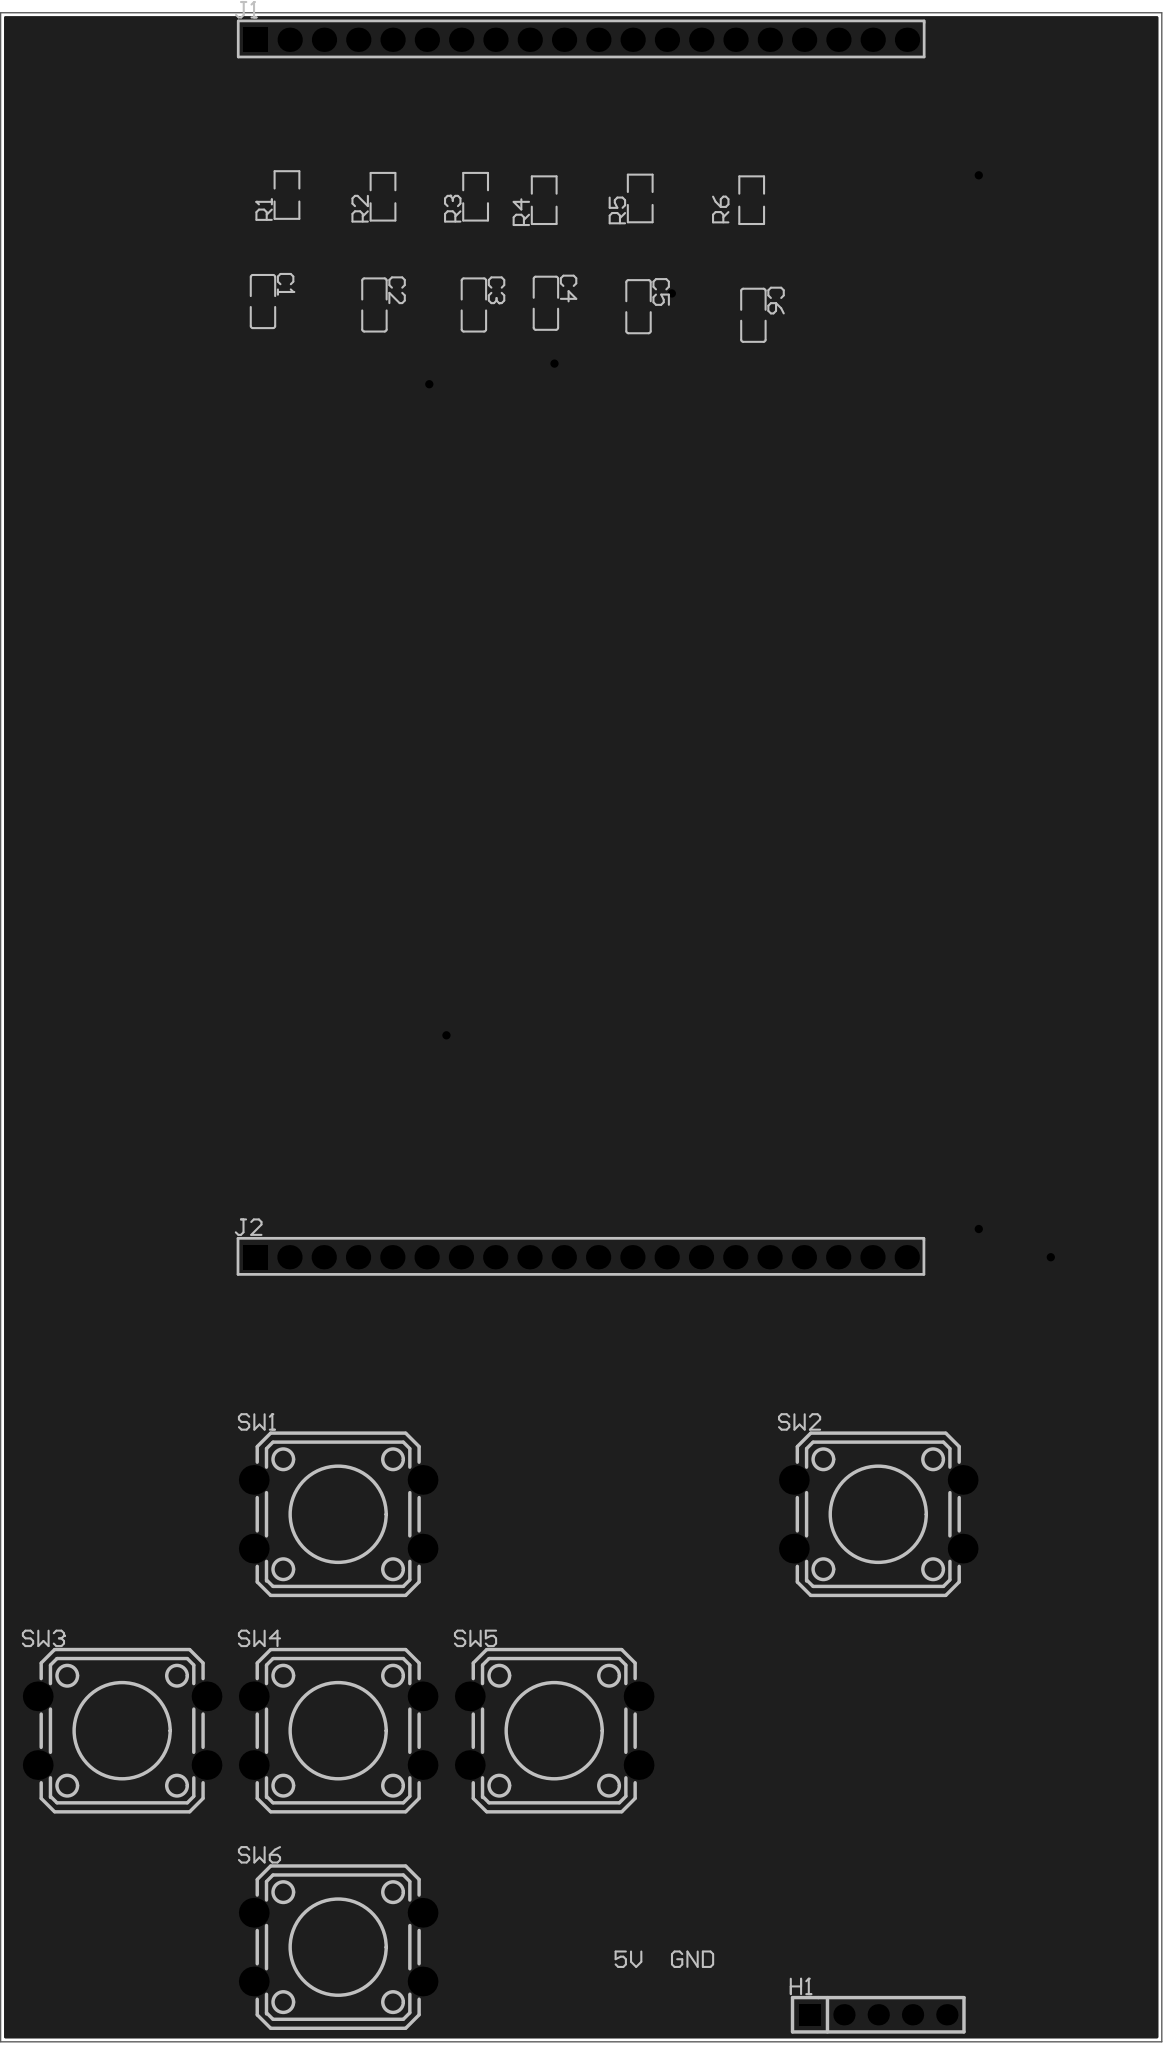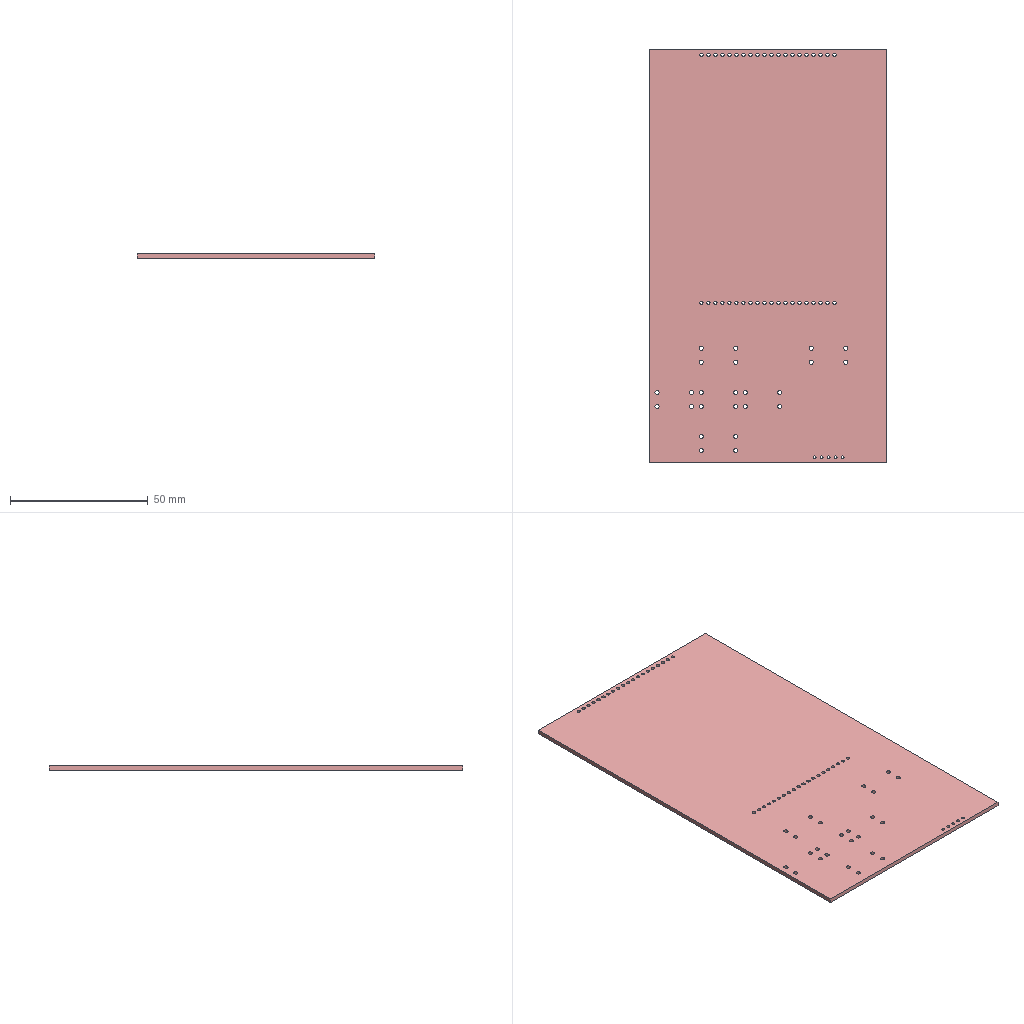Circuit board layout | Altium Designer | box 86 x 150 x 1.6 mm
Layer stack:
# Altium Designer layer stack of  (unit mm; dielectric type: 0 none, 1 core, 2 prepreg, 3 surface material)
index,name,kind,layer,copper_thickness_mm,dielectric_type,dielectric_thickness_mm,dielectric_material,dielectric_constant
0,Top Paste Mask Layer,other,,,,,,
1,Top Silkscreen Layer,other,,,,,,
2,Top Solder Mask Layer,dielectric,,,3,0.01,,3.3
3,Top Layer,copper,Top Layer,0.035,,,,
4,Dielectric1,dielectric,,,3,1.51,FR4,4.5
5,Bottom Layer,copper,Bottom Layer,0.035,,,,
6,Bottom Solder Mask Layer,dielectric,,,3,0.01,,3.3
7,Bottom Silkscreen Layer,other,,,,,,
8,Bottom Paste Mask Layer,other,,,,,,
# drill layer pairs: low layer,high layer
drill_pair,Top Layer,Bottom Layer
Part placement:
Designator,Comment,Layer,Footprint,Center-X(mm),Center-Y(mm),Rotation
5V,,TopLayer,Test-Point-0.5mm,152.042,103.874,0
C1,100nF,TopLayer,C0805,125.674,227.367,270
C2,100nF,TopLayer,C0805,133.929,227.113,270
C3,100nF,TopLayer,C0805,141.295,227.113,270
C4,100nF,TopLayer,C0805,146.629,227.24,270
C5,100nF,TopLayer,C0805,153.487,226.986,270
C6,100nF,TopLayer,C0805,161.996,226.351,270
GND,,TopLayer,Test-Point-0.5mm,156.217,103.874,0
H1,2.54-1*5P母,TopLayer,HDR-TH_5P-P2.54-V-F,171.243,100.716,0
J1,2.54-1*20P直针,TopLayer,HDR-TH_20P-P2.54-V-M-1,149.244,246.716,0
R1,10kΩ,TopLayer,R0805,127.452,235.241,90
R2,10kΩ,TopLayer,R0805,134.564,235.114,90
R3,10kΩ,TopLayer,R0805,141.422,235.114,90
R4,10kΩ,TopLayer,R0805,146.502,234.86,90
R5,10kΩ,TopLayer,R0805,153.614,234.987,90
R6,10kΩ,TopLayer,R0805,161.869,234.86,90
SW1,TC-1103-C-K,TopLayer,KEY-TH_4P-L12.0-W12.0-P5.00-LS12.5,131.243,137.716,0
SW2,TC-1103-C-K,TopLayer,KEY-TH_4P-L12.0-W12.0-P5.00-LS12.5,171.243,137.716,0
SW3,TC-1103-C-K,TopLayer,KEY-TH_4P-L12.0-W12.0-P5.00-LS12.5,115.243,121.716,0
SW4,TC-1103-C-K,TopLayer,KEY-TH_4P-L12.0-W12.0-P5.00-LS12.5,131.244,121.716,0
SW5,TC-1103-C-K,TopLayer,KEY-TH_4P-L12.0-W12.0-P5.00-LS12.5,147.243,121.716,0
SW6,TC-1103-C-K,TopLayer,KEY-TH_4P-L12.0-W12.0-P5.00-LS12.5,131.244,105.716,0
J2,2.54-1*20P直针,TopLayer,HDR-TH_20P-P2.54-V-M-1,149.225,156.718,0
Pad and via stacks:
# Altium Designer via and pad stacks of  (unit mm). Each distinct definition once, with the count of objects using it.
# via: kind,start_layer,end_layer,hole_mm,diameter_mm,mode(0 simple;1 top-mid-bottom;2 full stack),diameter_per_layer,count,example_net
# pad: kind,layer,hole_mm,hole_type(0 round;1 square;2 slot),plating,top_size,top_shape(1 round;2 rect;3 octagon;9 rounded rect),mid_size,bottom_size,mode,footprint,size_per_layer,count,example
pad,Top Layer,0,0,plated,0.5x0.5,1,0.5x0.5,0.5x0.5,0,Test-Point-0.5mm,,2,5V.1
pad,Top Layer,0,0,plated,1.41x1.35,2,1.41x1.35,1.41x1.35,0,C0805,,12,C1.2
pad,Top Layer,0,0,plated,1.133x1.377,2,1.133x1.377,1.133x1.377,0,R0805,,12,R1.2
pad,Multi-Layer,1.02,0,plated,1.575x1.575,1,1.575x1.575,1.575x1.575,0,HDR-TH_5P-P2.54-V-F,,4,H1.5
pad,Multi-Layer,1.02,0,plated,1.575x1.575,2,1.575x1.575,1.575x1.575,0,HDR-TH_5P-P2.54-V-F,,1,H1.1
pad,Multi-Layer,1.2,0,plated,1.8x1.8,1,1.8x1.8,1.8x1.8,0,HDR-TH_20P-P2.54-V-M-1,,38,J1.20
pad,Multi-Layer,1.2,0,plated,1.8x1.8,2,1.8x1.8,1.8x1.8,0,HDR-TH_20P-P2.54-V-M-1,,2,J1.1
pad,Multi-Layer,1.501,0,plated,2.2x2.2,1,2.2x2.2,2.2x2.2,0,KEY-TH_4P-L12.0-W12.0-P5.00-LS12.5,,24,SW1.1
via,Top Layer,Bottom Layer,0.3048,0.61,0,,7,$1N57
Copper pours:
name,layer,net,type(0 solid;1 hatched;2 none)
Top Layer-GND,Top Layer,GND,0
Bottom Layer-GND,Bottom Layer,GND,0